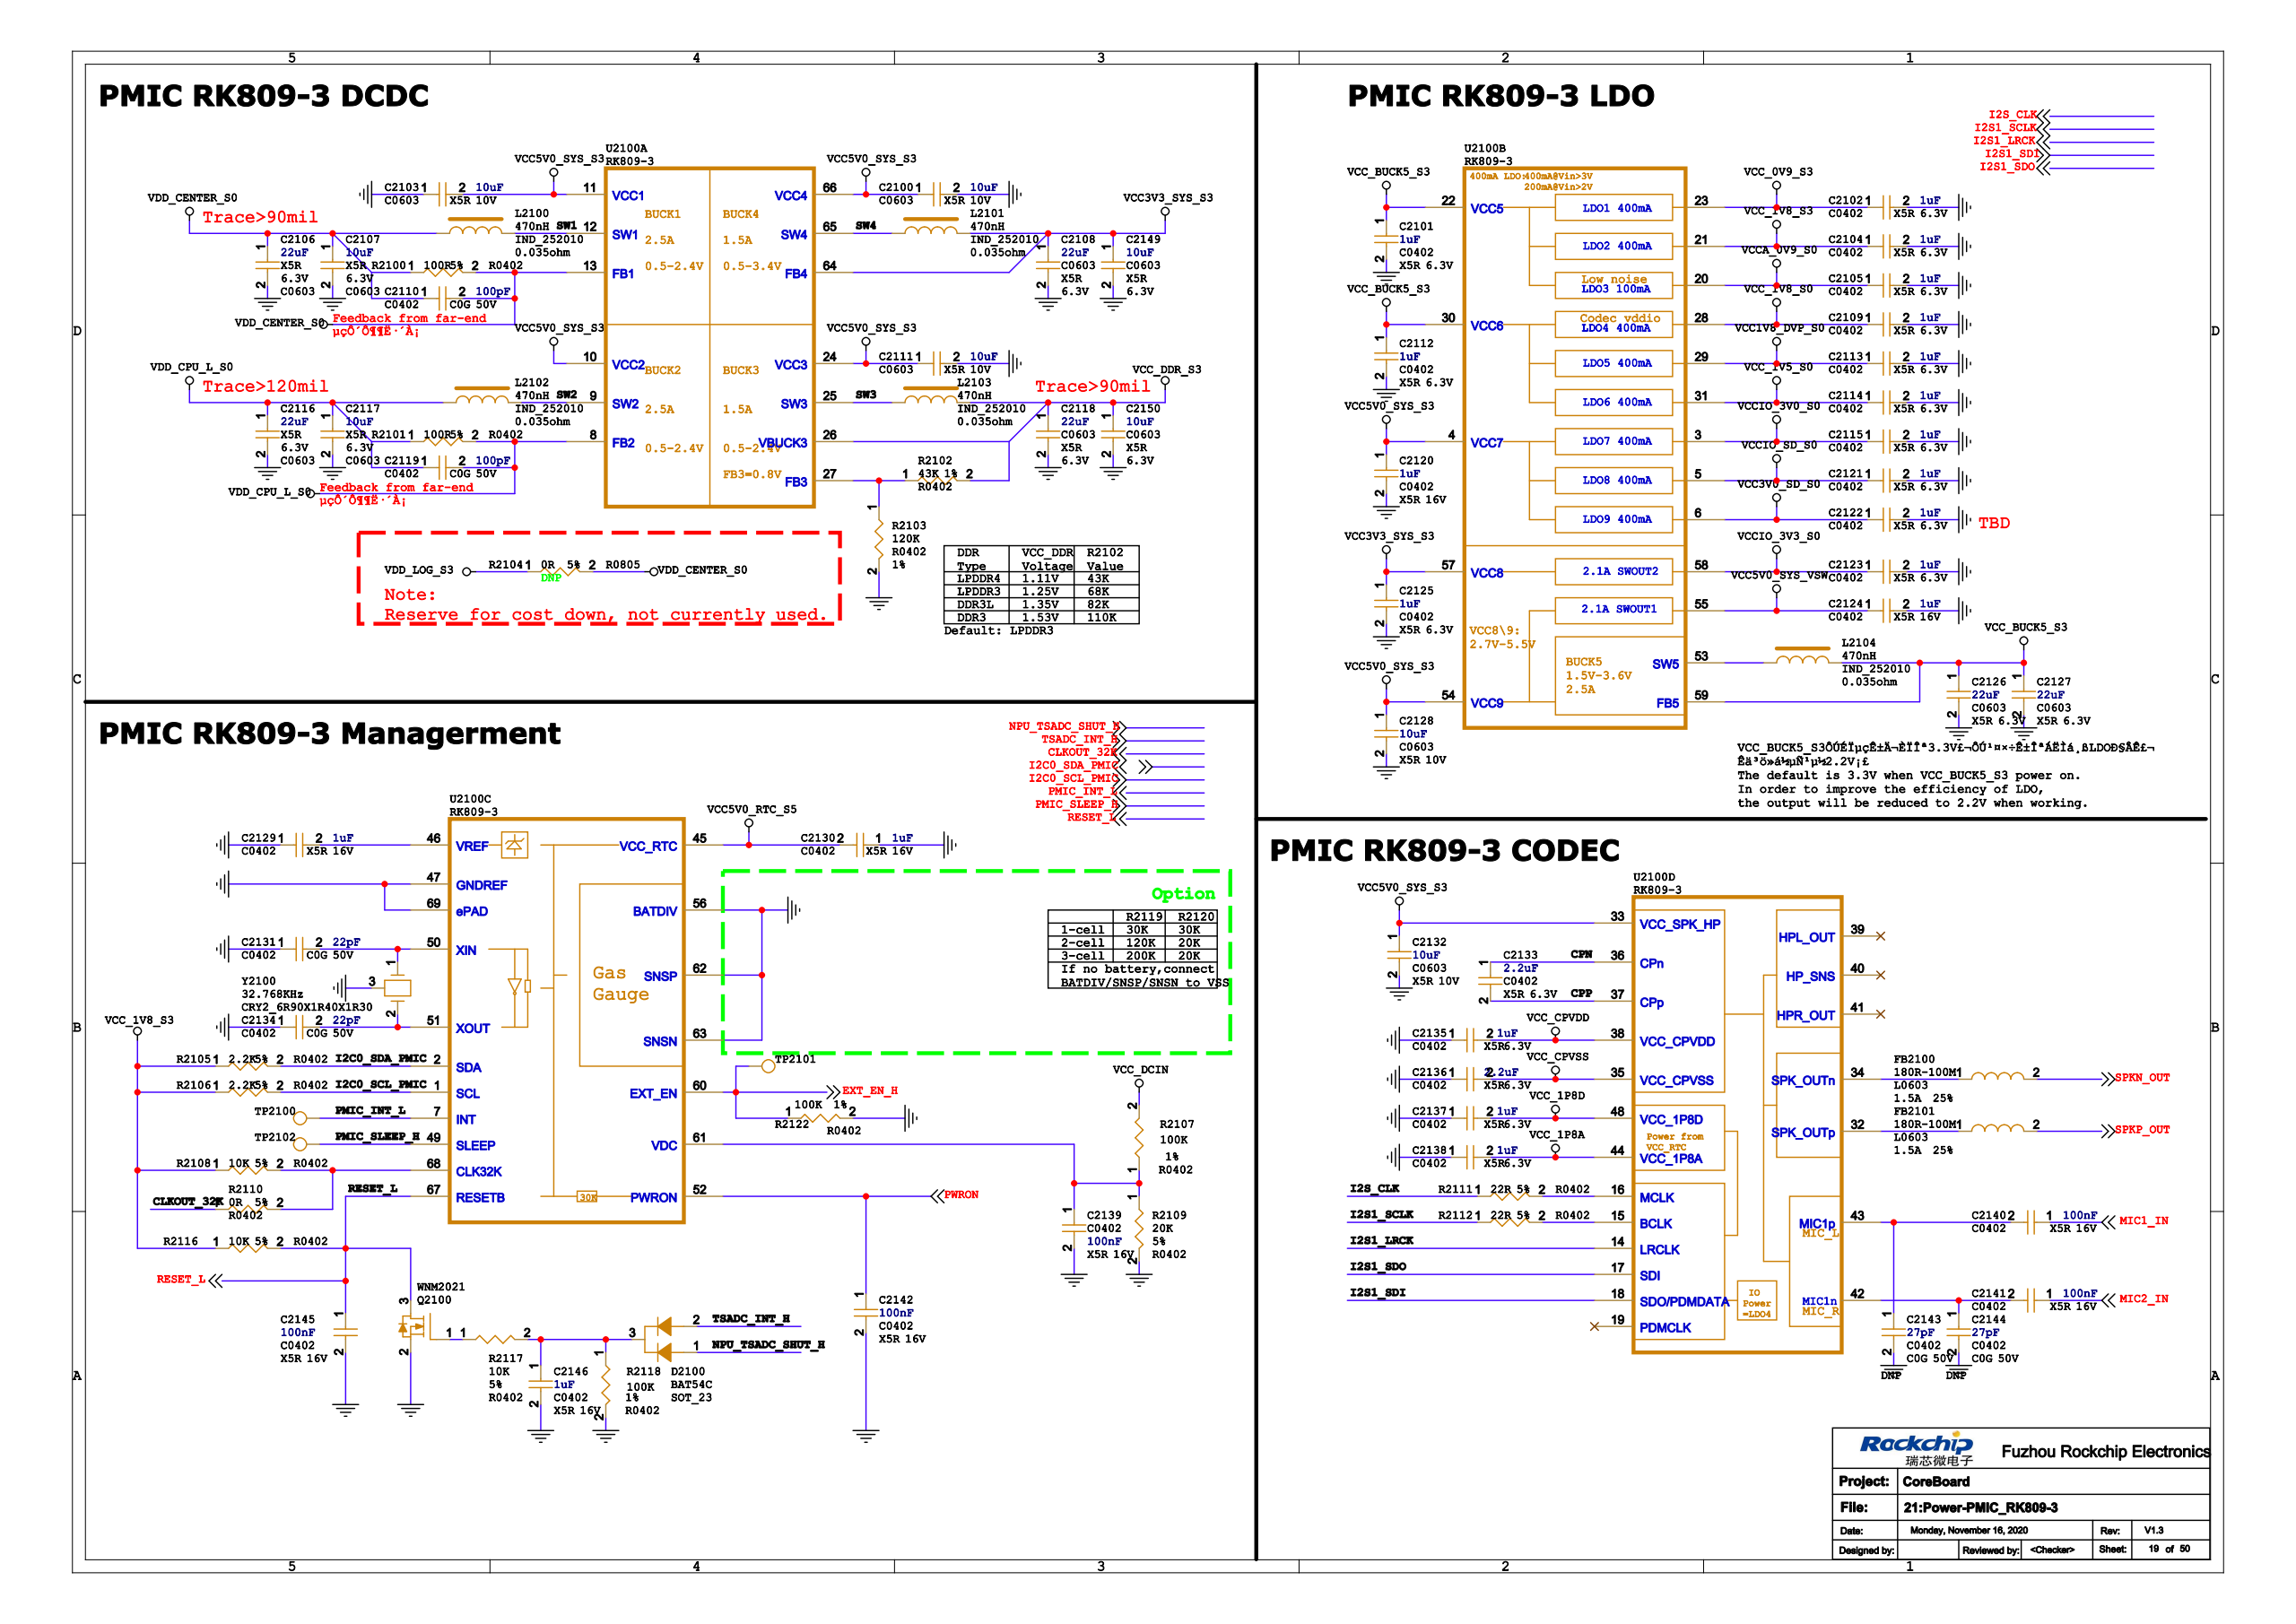Circuit board | Cadence Allegro | 749 parts | 717 nets | one sheet of the schematic
Parts on this sheet (reference | value | footprint):
C2100 | 10uF | C0603
C2101 | 1uF | C0402
C2102 | 1uF | C0402
C2103 | 10uF | C0603
C2104 | 1uF | C0402
C2105 | 1uF | C0402
C2106 | 22uF | C0603
C2107 | 10uF | C0603
C2108 | 22uF | C0603
C2109 | 1uF | C0402
C2110 | 100pF | C0402
C2111 | 10uF | C0603
C2112 | 1uF | C0402
C2113 | 1uF | C0402
C2114 | 1uF | C0402
C2115 | 1uF | C0402
C2116 | 22uF | C0603
C2117 | 10uF | C0603
C2118 | 22uF | C0603
C2119 | 100pF | C0402
C2120 | 1uF | C0402
C2121 | 1uF | C0402
C2122 | 1uF | C0402
C2123 | 1uF | C0402
C2124 | 1uF | C0402
C2125 | 1uF | C0402
C2126 | 22uF | C0603
C2127 | 22uF | C0603
C2128 | 10uF | C0603
C2129 | 1uF | C0402
C2130 | 1uF | C0402
C2131 | 22pF | C0402
C2132 | 10uF | C0603
C2133 | 2.2uF | C0402
C2134 | 22pF | C0402
C2135 | 1uF | C0402
C2136 | 2.2uF | C0402
C2137 | 1uF | C0402
C2138 | 1uF | C0402
C2139 | 100nF | C0402
C2140 | 100nF | C0402
C2141 | 100nF | C0402
C2142 | 100nF | C0402
C2143 | 27pF | C0402
C2144 | 27pF | C0402
C2145 | 100nF | C0402
C2146 | 1uF | C0402
C2149 | 10uF | C0603
C2150 | 10uF | C0603
D2100 | BAT54C | SOT_23
FB2100 | 180R-100M | L0603
FB2101 | 180R-100M | L0603
L2100 | 470nH | IND_252010
L2101 | 470nH | IND_252010
L2102 | 470nH | IND_252010
L2103 | 470nH | IND_252010
L2104 | 470nH | IND_252010
Q2100 | WNM2021 | SOT_323
R2102 | 43K | R0402
R2103 | 120K | R0402
R2104 | 0R | R0805
R2107 | 100K | R0402
R2109 | 20K | R0402
R2110 | 0R | R0402
R2116 | 10K | R0402
R2117 | 10K | R0402
R2118 | 100K | R0402
R2122 | 100K | R0402
TP2100 | TP_0.7 | TP_0R70
TP2101 | TP_0.7 | TP_0R70
TP2102 | TP_0.7 | TP_0R70
U2100 | RK809-3 | QFN68_7R00X7R00X0R80_T
Y2100 | 32.768KHz | CRY2_6R90X1R40X1R30
Nets of these parts (net: part-pin ...):
GND: C2100-2 C2101-2 C2102-2 C2103-1 C2104-2 C2105-2 C2106-2 C2107-2 C2108-2 C2109-2 C2111-2 C2112-2 C2113-2 C2114-2 C2115-2 C2116-2 C2117-2 C2118-2 C2120-2 C2121-2 C2122-2 C2123-2 C2124-2 C2125-2 C2126-2 C2127-2 C2128-2 C2129-1 C2130-1 C2131-1 C2132-2 C2134-1 C2135-1 C2136-1 C2137-1 C2138-1 C2139-2 C2142-2 C2143-2 C2144-2 C2145-2 C2146-2 C2149-2 C2150-2 Q2100-2 R2103-2 R2109-2 R2118-2 R2122-2 Y2100-3 U2100-47 U2100-56 U2100-62 U2100-63 U2100-69
VCC_1V8_S0: C2109-1 U2100-28
VCC_DCIN: R2107-2
RESET_L: C2145-1 Q2100-3 R2116-2 U2100-67
CLKOUT_32K: R2110-1
MIC1_IN: C2140-1
SPKN_OUT: FB2100-2
SPKP_OUT: FB2101-2
PWRON: C2142-1 U2100-52
VCC5V0_SYS_VSW: C2124-1 U2100-55
VCC5V0_SYS_S3: C2100-1 C2103-2 C2111-1 C2120-1 C2128-1 C2132-1 U2100-4 U2100-10 U2100-11 U2100-24 U2100-33 U2100-54 U2100-66
VCCIO_3V3_S0: C2123-1 U2100-58
VCC3V3_SYS_S3: C2108-1 C2125-1 C2149-1 L2101-2 U2100-57 U2100-64
VCCIO_3V0_S0: C2115-1 U2100-3
N16900970: Q2100-1 R2117-1
N17445677: R2102-1 R2103-1 U2100-27
VCC_DDR_S3: C2118-1 C2150-1 L2103-2 R2102-2 U2100-26
N83607440: C2131-2 Y2100-1 U2100-50
N83607438: C2134-2 Y2100-2 U2100-51
VDD_LOG_S3: R2104-1
VDD_CENTER_S0: C2106-1 C2107-1 C2110-1 C2110-2 L2100-2 R2104-2 U2100-13
VDD_CPU_L_S0: C2116-1 C2117-1 C2119-1 C2119-2 L2102-2 U2100-8
CPN: C2133-1 U2100-36
CPP: C2133-2 U2100-37
VCC_CPVSS: C2136-2 U2100-35
N17505600: C2140-2 C2143-1 U2100-43
N17505458: C2141-2 C2144-1 U2100-42
VCC_BUCK5_S3: C2101-1 C2112-1 C2126-1 C2127-1 L2104-1 U2100-22 U2100-30 U2100-59
NPU_TSADC_SHUT_H: D2100-1
TSADC_INT_H: D2100-2
N83607377: C2146-1 D2100-3 R2117-2 R2118-1
N17505520: FB2100-1 U2100-34
N17505530: FB2101-1 U2100-32
SW1: L2100-1 U2100-12
SW4: L2101-1 U2100-65
SW2: L2102-1 U2100-9
SW3: L2103-1 U2100-25
N77245547: L2104-2 U2100-53
N83607369: C2139-1 R2107-1 R2109-1 U2100-61
EXT_EN_H: R2122-1 TP2101-1 U2100-60
VCC5V0_RTC_S5: C2130-2 U2100-45
VCC_1V8_S3: C2104-1 R2116-1 U2100-21
VCC_0V9_S3: C2102-1 U2100-23
PMIC_SLEEP_H: TP2102-1 U2100-49
PMIC_INT_L: TP2100-1 U2100-7
I2C0_SDA_PMIC: U2100-2
I2C0_SCL_PMIC: U2100-1
VCCA_0V9_S0: C2105-1 U2100-20
VCC_1V5_S0: C2114-1 U2100-31
I2S1_LRCK: U2100-14
I2S1_SDI: U2100-18
I2S1_SDO: U2100-17
VCC1V8_DVP_S0: C2113-1 U2100-29
VCCIO_SD_S0: C2121-1 U2100-5
VCC3V0_SD_S0: C2122-1 U2100-6
N83607547: R2110-2 U2100-68
N83607432: C2129-2 U2100-46
VCC_1P8A: C2138-2 U2100-44
VCC_1P8D: C2137-2 U2100-48
VCC_CPVDD: C2135-2 U2100-38
MIC2_IN: C2141-1